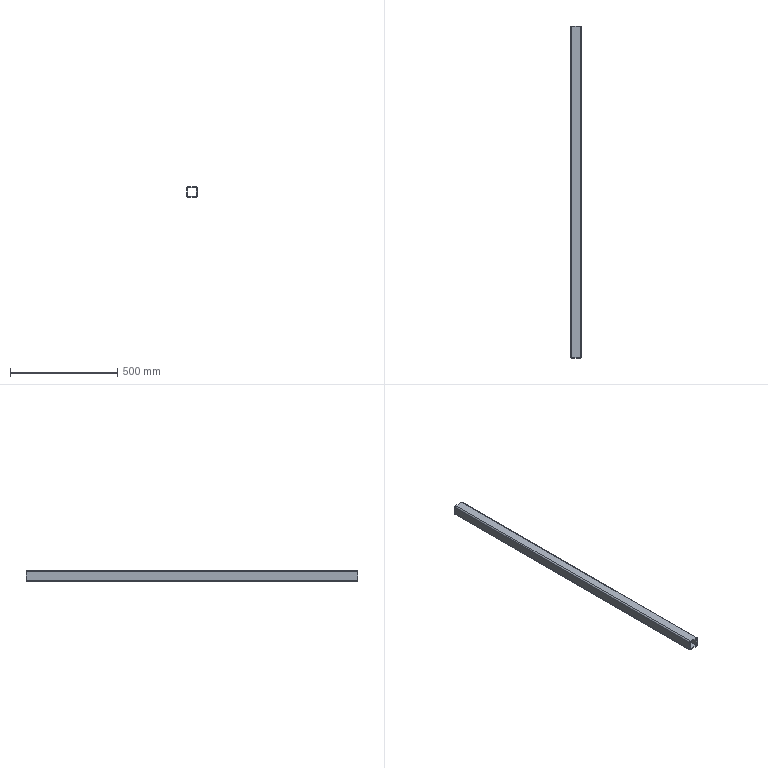Part | SolidWorks | features ICE 4, Extrusion 1 | 1 solid | 80 faces | box 50 x 1550 x 50 mm | volume 1299737 mm3 | cylinder 70 | plane 10 | commonest cylinder face diameters 20 x62 2 x4 12 x4